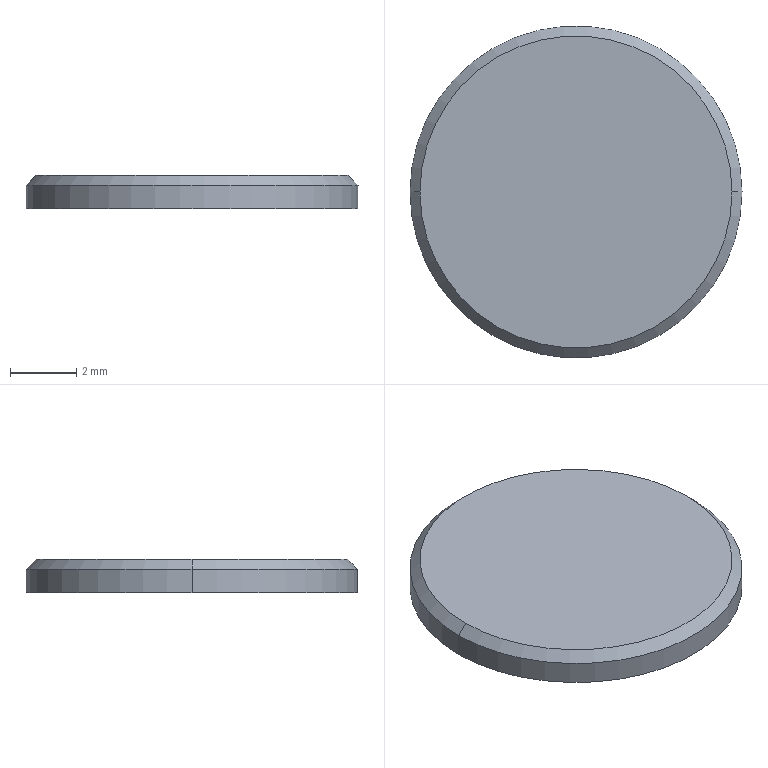Part | STEP file | 1 solid | 6 faces | box 10 x 10 x 1 mm | volume 77.154 mm3 | cylinder 2 | cone 2 | plane 2 | commonest cylinder face diameters 10 x2
STEP:
#1=CARTESIAN_POINT('',(-5.,0.,0.7));
#2=VERTEX_POINT('',#1);
#3=CARTESIAN_POINT('',(5.,0.,0.7));
#4=VERTEX_POINT('',#3);
#5=CARTESIAN_POINT('',(0.,0.,0.7));
#6=DIRECTION('',(0.,0.,-1.));
#7=DIRECTION('',(-1.,0.,0.));
#8=AXIS2_PLACEMENT_3D('',#5,#6,#7);
#9=CIRCLE('',#8,5.);
#10=EDGE_CURVE('',#2,#4,#9,.T.);
#11=ORIENTED_EDGE('',*,*,#10,.T.);
#12=CARTESIAN_POINT('',(5.,0.,0.));
#13=VERTEX_POINT('',#12);
#14=CARTESIAN_POINT('',(5.,0.,1.));
#15=DIRECTION('',(0.,0.,-1.));
#16=VECTOR('',#15,1000.);
#17=LINE('',#14,#16);
#18=EDGE_CURVE('',#4,#13,#17,.T.);
#19=ORIENTED_EDGE('',*,*,#18,.T.);
#20=CARTESIAN_POINT('',(-5.,0.,0.));
#21=VERTEX_POINT('',#20);
#22=CARTESIAN_POINT('',(0.,0.,0.));
#23=DIRECTION('',(0.,0.,1.));
#24=DIRECTION('',(-1.,0.,0.));
#25=AXIS2_PLACEMENT_3D('',#22,#23,#24);
#26=CIRCLE('',#25,5.);
#27=EDGE_CURVE('',#13,#21,#26,.T.);
#28=ORIENTED_EDGE('',*,*,#27,.T.);
#29=CARTESIAN_POINT('',(-5.,0.,1.));
#30=DIRECTION('',(0.,0.,-1.));
#31=VECTOR('',#30,1000.);
#32=LINE('',#29,#31);
#33=EDGE_CURVE('',#2,#21,#32,.T.);
#34=ORIENTED_EDGE('',*,*,#33,.F.);
#35=EDGE_LOOP('',(#11,#19,#28,#34));
#36=FACE_OUTER_BOUND('',#35,.T.);
#37=CARTESIAN_POINT('',(0.,0.,1.));
#38=DIRECTION('',(0.,0.,-1.));
#39=DIRECTION('',(-1.,0.,0.));
#40=AXIS2_PLACEMENT_3D('',#37,#38,#39);
#41=CYLINDRICAL_SURFACE('',#40,5.);
#42=ADVANCED_FACE('',(#36),#41,.T.);
#43=CARTESIAN_POINT('',(-4.7,0.,1.));
#44=VERTEX_POINT('',#43);
#45=CARTESIAN_POINT('',(4.7,0.,1.));
#46=VERTEX_POINT('',#45);
#47=CARTESIAN_POINT('',(0.,0.,1.));
#48=DIRECTION('',(0.,0.,-1.));
#49=DIRECTION('',(-1.,0.,0.));
#50=AXIS2_PLACEMENT_3D('',#47,#48,#49);
#51=CIRCLE('',#50,4.7);
#52=EDGE_CURVE('',#44,#46,#51,.T.);
#53=ORIENTED_EDGE('',*,*,#52,.T.);
#54=CARTESIAN_POINT('',(5.,0.,0.7));
#55=DIRECTION('',(0.7071,0.,-0.7071));
#56=VECTOR('',#55,1000.);
#57=LINE('',#54,#56);
#58=EDGE_CURVE('',#46,#4,#57,.T.);
#59=ORIENTED_EDGE('',*,*,#58,.T.);
#60=ORIENTED_EDGE('',*,*,#10,.F.);
#61=CARTESIAN_POINT('',(-5.,0.,0.7));
#62=DIRECTION('',(-0.7071,0.,-0.7071));
#63=VECTOR('',#62,1000.);
#64=LINE('',#61,#63);
#65=EDGE_CURVE('',#44,#2,#64,.T.);
#66=ORIENTED_EDGE('',*,*,#65,.F.);
#67=EDGE_LOOP('',(#53,#59,#60,#66));
#68=FACE_OUTER_BOUND('',#67,.T.);
#69=CARTESIAN_POINT('',(0.,0.,0.7));
#70=DIRECTION('',(0.,0.,-1.));
#71=DIRECTION('',(-1.,0.,0.));
#72=AXIS2_PLACEMENT_3D('',#69,#70,#71);
#73=CONICAL_SURFACE('',#72,5.,0.7854);
#74=ADVANCED_FACE('',(#68),#73,.T.);
#75=CARTESIAN_POINT('',(0.,0.,0.));
#76=DIRECTION('',(0.,0.,1.));
#77=DIRECTION('',(-1.,0.,0.));
#78=AXIS2_PLACEMENT_3D('',#75,#76,#77);
#79=CIRCLE('',#78,5.);
#80=EDGE_CURVE('',#21,#13,#79,.T.);
#81=ORIENTED_EDGE('',*,*,#80,.F.);
#82=ORIENTED_EDGE('',*,*,#27,.F.);
#83=EDGE_LOOP('',(#81,#82));
#84=FACE_OUTER_BOUND('',#83,.T.);
#85=CARTESIAN_POINT('',(0.,0.,0.));
#86=DIRECTION('',(0.,0.,1.));
#87=DIRECTION('',(1.,0.,0.));
#88=AXIS2_PLACEMENT_3D('',#85,#86,#87);
#89=PLANE('',#88);
#90=ADVANCED_FACE('',(#84),#89,.F.);
#91=ORIENTED_EDGE('',*,*,#18,.F.);
#92=CARTESIAN_POINT('',(0.,0.,0.7));
#93=DIRECTION('',(0.,0.,-1.));
#94=DIRECTION('',(-1.,0.,0.));
#95=AXIS2_PLACEMENT_3D('',#92,#93,#94);
#96=CIRCLE('',#95,5.);
#97=EDGE_CURVE('',#4,#2,#96,.T.);
#98=ORIENTED_EDGE('',*,*,#97,.T.);
#99=ORIENTED_EDGE('',*,*,#33,.T.);
#100=ORIENTED_EDGE('',*,*,#80,.T.);
#101=EDGE_LOOP('',(#91,#98,#99,#100));
#102=FACE_OUTER_BOUND('',#101,.T.);
#103=CARTESIAN_POINT('',(0.,0.,1.));
#104=DIRECTION('',(0.,0.,-1.));
#105=DIRECTION('',(-1.,0.,0.));
#106=AXIS2_PLACEMENT_3D('',#103,#104,#105);
#107=CYLINDRICAL_SURFACE('',#106,5.);
#108=ADVANCED_FACE('',(#102),#107,.T.);
#109=ORIENTED_EDGE('',*,*,#58,.F.);
#110=CARTESIAN_POINT('',(0.,0.,1.));
#111=DIRECTION('',(0.,0.,-1.));
#112=DIRECTION('',(-1.,0.,0.));
#113=AXIS2_PLACEMENT_3D('',#110,#111,#112);
#114=CIRCLE('',#113,4.7);
#115=EDGE_CURVE('',#46,#44,#114,.T.);
#116=ORIENTED_EDGE('',*,*,#115,.T.);
#117=ORIENTED_EDGE('',*,*,#65,.T.);
#118=ORIENTED_EDGE('',*,*,#97,.F.);
#119=EDGE_LOOP('',(#109,#116,#117,#118));
#120=FACE_OUTER_BOUND('',#119,.T.);
#121=CARTESIAN_POINT('',(0.,0.,0.7));
#122=DIRECTION('',(0.,0.,-1.));
#123=DIRECTION('',(-1.,0.,0.));
#124=AXIS2_PLACEMENT_3D('',#121,#122,#123);
#125=CONICAL_SURFACE('',#124,5.,0.7854);
#126=ADVANCED_FACE('',(#120),#125,.T.);
#127=ORIENTED_EDGE('',*,*,#52,.F.);
#128=ORIENTED_EDGE('',*,*,#115,.F.);
#129=EDGE_LOOP('',(#127,#128));
#130=FACE_OUTER_BOUND('',#129,.T.);
#131=CARTESIAN_POINT('',(0.,0.,1.));
#132=DIRECTION('',(0.,0.,1.));
#133=DIRECTION('',(1.,0.,0.));
#134=AXIS2_PLACEMENT_3D('',#131,#132,#133);
#135=PLANE('',#134);
#136=ADVANCED_FACE('',(#130),#135,.T.);
#137=CLOSED_SHELL('',(#42,#74,#90,#108,#126,#136));
#138=MANIFOLD_SOLID_BREP('',#137);
#139=CARTESIAN_POINT('',(0.,0.,0.));
#140=DIRECTION('',(0.,0.,1.));
#141=DIRECTION('',(1.,0.,0.));
#142=AXIS2_PLACEMENT_3D('',#139,#140,#141);
#143=(LENGTH_UNIT()NAMED_UNIT(*)SI_UNIT(.MILLI.,.METRE.));
#144=UNCERTAINTY_MEASURE_WITH_UNIT(LENGTH_MEASURE(0.00001),#143,'','');
#145=(NAMED_UNIT(*)PLANE_ANGLE_UNIT()SI_UNIT($,.RADIAN.));
#146=(NAMED_UNIT(*)SI_UNIT($,.STERADIAN.)SOLID_ANGLE_UNIT());
#147=(GEOMETRIC_REPRESENTATION_CONTEXT(3)GLOBAL_UNCERTAINTY_ASSIGNED_CONTEXT((#144))GLOBAL_UNIT_ASSIGNED_CONTEXT((#143,#145,#146))REPRESENTATION_CONTEXT('',''));
#148=ADVANCED_BREP_SHAPE_REPRESENTATION('',(#138,#142),#147);